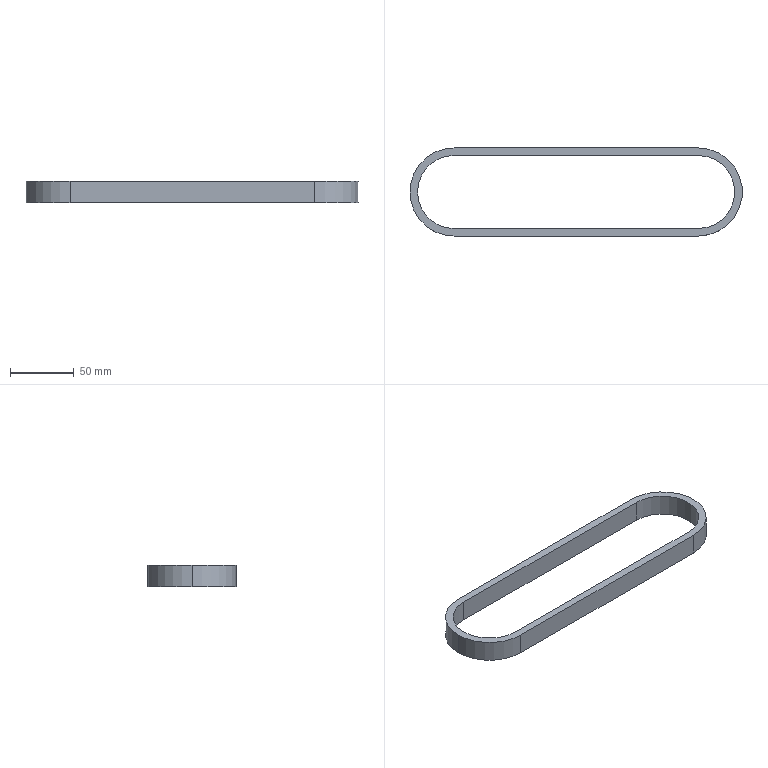Part | SolidWorks | features BaseBody 1 | 1 solid | 12 faces | box 259.87 x 68.87 x 17 mm | volume 58157 mm3 | cylinder 6 | plane 6 | commonest cylinder face diameters 57.07 x3 68.87 x3
STEP:
#1=CARTESIAN_POINT('',(0.,28.535,17.));
#2=VERTEX_POINT('',#1);
#3=CARTESIAN_POINT('',(-28.535,0.,17.));
#4=VERTEX_POINT('',#3);
#5=CARTESIAN_POINT('',(0.,0.,17.));
#6=DIRECTION('',(0.,0.,1.));
#7=DIRECTION('',(1.,0.,0.));
#8=AXIS2_PLACEMENT_3D('',#5,#6,#7);
#9=CIRCLE('',#8,28.535);
#10=EDGE_CURVE('',#2,#4,#9,.T.);
#11=ORIENTED_EDGE('',*,*,#10,.T.);
#12=CARTESIAN_POINT('',(-28.535,0.,0.));
#13=VERTEX_POINT('',#12);
#14=CARTESIAN_POINT('',(-28.535,0.,17.));
#15=DIRECTION('',(0.,0.,-1.));
#16=VECTOR('',#15,1000.);
#17=LINE('',#14,#16);
#18=EDGE_CURVE('',#4,#13,#17,.T.);
#19=ORIENTED_EDGE('',*,*,#18,.T.);
#20=CARTESIAN_POINT('',(0.,28.535,0.));
#21=VERTEX_POINT('',#20);
#22=CARTESIAN_POINT('',(0.,0.,0.));
#23=DIRECTION('',(0.,0.,1.));
#24=DIRECTION('',(1.,0.,0.));
#25=AXIS2_PLACEMENT_3D('',#22,#23,#24);
#26=CIRCLE('',#25,28.535);
#27=EDGE_CURVE('',#21,#13,#26,.T.);
#28=ORIENTED_EDGE('',*,*,#27,.F.);
#29=CARTESIAN_POINT('',(0.,28.535,17.));
#30=DIRECTION('',(0.,0.,-1.));
#31=VECTOR('',#30,1000.);
#32=LINE('',#29,#31);
#33=EDGE_CURVE('',#2,#21,#32,.T.);
#34=ORIENTED_EDGE('',*,*,#33,.F.);
#35=EDGE_LOOP('',(#11,#19,#28,#34));
#36=FACE_OUTER_BOUND('',#35,.T.);
#37=CARTESIAN_POINT('',(0.,0.,17.));
#38=DIRECTION('',(0.,0.,-1.));
#39=DIRECTION('',(-1.,0.,0.));
#40=AXIS2_PLACEMENT_3D('',#37,#38,#39);
#41=CYLINDRICAL_SURFACE('',#40,28.535);
#42=ADVANCED_FACE('',(#36),#41,.F.);
#43=CARTESIAN_POINT('',(-34.435,0.,17.));
#44=VERTEX_POINT('',#43);
#45=CARTESIAN_POINT('',(0.,-34.435,17.));
#46=VERTEX_POINT('',#45);
#47=CARTESIAN_POINT('',(0.,0.,17.));
#48=DIRECTION('',(0.,0.,1.));
#49=DIRECTION('',(1.,0.,0.));
#50=AXIS2_PLACEMENT_3D('',#47,#48,#49);
#51=CIRCLE('',#50,34.435);
#52=EDGE_CURVE('',#44,#46,#51,.T.);
#53=ORIENTED_EDGE('',*,*,#52,.F.);
#54=CARTESIAN_POINT('',(-34.435,0.,0.));
#55=VERTEX_POINT('',#54);
#56=CARTESIAN_POINT('',(-34.435,0.,17.));
#57=DIRECTION('',(0.,0.,-1.));
#58=VECTOR('',#57,1000.);
#59=LINE('',#56,#58);
#60=EDGE_CURVE('',#44,#55,#59,.T.);
#61=ORIENTED_EDGE('',*,*,#60,.T.);
#62=CARTESIAN_POINT('',(0.,-34.435,0.));
#63=VERTEX_POINT('',#62);
#64=CARTESIAN_POINT('',(0.,0.,0.));
#65=DIRECTION('',(0.,0.,1.));
#66=DIRECTION('',(1.,0.,0.));
#67=AXIS2_PLACEMENT_3D('',#64,#65,#66);
#68=CIRCLE('',#67,34.435);
#69=EDGE_CURVE('',#55,#63,#68,.T.);
#70=ORIENTED_EDGE('',*,*,#69,.T.);
#71=CARTESIAN_POINT('',(0.,-34.435,17.));
#72=DIRECTION('',(0.,0.,-1.));
#73=VECTOR('',#72,1000.);
#74=LINE('',#71,#73);
#75=EDGE_CURVE('',#46,#63,#74,.T.);
#76=ORIENTED_EDGE('',*,*,#75,.F.);
#77=EDGE_LOOP('',(#53,#61,#70,#76));
#78=FACE_OUTER_BOUND('',#77,.T.);
#79=CARTESIAN_POINT('',(0.,0.,17.));
#80=DIRECTION('',(0.,0.,-1.));
#81=DIRECTION('',(-1.,0.,0.));
#82=AXIS2_PLACEMENT_3D('',#79,#80,#81);
#83=CYLINDRICAL_SURFACE('',#82,34.435);
#84=ADVANCED_FACE('',(#78),#83,.T.);
#85=CARTESIAN_POINT('',(0.,34.435,17.));
#86=VERTEX_POINT('',#85);
#87=CARTESIAN_POINT('',(0.,0.,17.));
#88=DIRECTION('',(0.,0.,1.));
#89=DIRECTION('',(1.,0.,0.));
#90=AXIS2_PLACEMENT_3D('',#87,#88,#89);
#91=CIRCLE('',#90,34.435);
#92=EDGE_CURVE('',#86,#44,#91,.T.);
#93=ORIENTED_EDGE('',*,*,#92,.T.);
#94=ORIENTED_EDGE('',*,*,#52,.T.);
#95=CARTESIAN_POINT('',(191.,-34.435,17.));
#96=VERTEX_POINT('',#95);
#97=CARTESIAN_POINT('',(0.,-34.435,17.));
#98=DIRECTION('',(1.,0.,0.));
#99=VECTOR('',#98,1000.);
#100=LINE('',#97,#99);
#101=EDGE_CURVE('',#46,#96,#100,.T.);
#102=ORIENTED_EDGE('',*,*,#101,.T.);
#103=CARTESIAN_POINT('',(191.,34.435,17.));
#104=VERTEX_POINT('',#103);
#105=CARTESIAN_POINT('',(191.,0.,17.));
#106=DIRECTION('',(0.,0.,1.));
#107=DIRECTION('',(1.,0.,0.));
#108=AXIS2_PLACEMENT_3D('',#105,#106,#107);
#109=CIRCLE('',#108,34.435);
#110=EDGE_CURVE('',#96,#104,#109,.T.);
#111=ORIENTED_EDGE('',*,*,#110,.T.);
#112=CARTESIAN_POINT('',(0.,34.435,17.));
#113=DIRECTION('',(-1.,0.,0.));
#114=VECTOR('',#113,1000.);
#115=LINE('',#112,#114);
#116=EDGE_CURVE('',#104,#86,#115,.T.);
#117=ORIENTED_EDGE('',*,*,#116,.T.);
#118=EDGE_LOOP('',(#93,#94,#102,#111,#117));
#119=FACE_OUTER_BOUND('',#118,.T.);
#120=CARTESIAN_POINT('',(0.,-28.535,17.));
#121=VERTEX_POINT('',#120);
#122=CARTESIAN_POINT('',(191.,-28.535,17.));
#123=VERTEX_POINT('',#122);
#124=CARTESIAN_POINT('',(0.,-28.535,17.));
#125=DIRECTION('',(1.,0.,0.));
#126=VECTOR('',#125,1000.);
#127=LINE('',#124,#126);
#128=EDGE_CURVE('',#121,#123,#127,.T.);
#129=ORIENTED_EDGE('',*,*,#128,.F.);
#130=CARTESIAN_POINT('',(0.,0.,17.));
#131=DIRECTION('',(0.,0.,1.));
#132=DIRECTION('',(1.,0.,0.));
#133=AXIS2_PLACEMENT_3D('',#130,#131,#132);
#134=CIRCLE('',#133,28.535);
#135=EDGE_CURVE('',#4,#121,#134,.T.);
#136=ORIENTED_EDGE('',*,*,#135,.F.);
#137=ORIENTED_EDGE('',*,*,#10,.F.);
#138=CARTESIAN_POINT('',(191.,28.535,17.));
#139=VERTEX_POINT('',#138);
#140=CARTESIAN_POINT('',(0.,28.535,17.));
#141=DIRECTION('',(-1.,0.,0.));
#142=VECTOR('',#141,1000.);
#143=LINE('',#140,#142);
#144=EDGE_CURVE('',#139,#2,#143,.T.);
#145=ORIENTED_EDGE('',*,*,#144,.F.);
#146=CARTESIAN_POINT('',(191.,0.,17.));
#147=DIRECTION('',(0.,0.,1.));
#148=DIRECTION('',(1.,0.,0.));
#149=AXIS2_PLACEMENT_3D('',#146,#147,#148);
#150=CIRCLE('',#149,28.535);
#151=EDGE_CURVE('',#123,#139,#150,.T.);
#152=ORIENTED_EDGE('',*,*,#151,.F.);
#153=EDGE_LOOP('',(#129,#136,#137,#145,#152));
#154=FACE_BOUND('',#153,.T.);
#155=CARTESIAN_POINT('',(0.,0.,17.));
#156=DIRECTION('',(0.,0.,1.));
#157=DIRECTION('',(1.,0.,0.));
#158=AXIS2_PLACEMENT_3D('',#155,#156,#157);
#159=PLANE('',#158);
#160=ADVANCED_FACE('',(#119,#154),#159,.T.);
#161=CARTESIAN_POINT('',(0.,34.435,0.));
#162=VERTEX_POINT('',#161);
#163=CARTESIAN_POINT('',(0.,0.,0.));
#164=DIRECTION('',(0.,0.,1.));
#165=DIRECTION('',(1.,0.,0.));
#166=AXIS2_PLACEMENT_3D('',#163,#164,#165);
#167=CIRCLE('',#166,34.435);
#168=EDGE_CURVE('',#162,#55,#167,.T.);
#169=ORIENTED_EDGE('',*,*,#168,.F.);
#170=CARTESIAN_POINT('',(191.,34.435,0.));
#171=VERTEX_POINT('',#170);
#172=CARTESIAN_POINT('',(0.,34.435,0.));
#173=DIRECTION('',(-1.,0.,0.));
#174=VECTOR('',#173,1000.);
#175=LINE('',#172,#174);
#176=EDGE_CURVE('',#171,#162,#175,.T.);
#177=ORIENTED_EDGE('',*,*,#176,.F.);
#178=CARTESIAN_POINT('',(191.,-34.435,0.));
#179=VERTEX_POINT('',#178);
#180=CARTESIAN_POINT('',(191.,0.,0.));
#181=DIRECTION('',(0.,0.,1.));
#182=DIRECTION('',(1.,0.,0.));
#183=AXIS2_PLACEMENT_3D('',#180,#181,#182);
#184=CIRCLE('',#183,34.435);
#185=EDGE_CURVE('',#179,#171,#184,.T.);
#186=ORIENTED_EDGE('',*,*,#185,.F.);
#187=CARTESIAN_POINT('',(0.,-34.435,0.));
#188=DIRECTION('',(1.,0.,0.));
#189=VECTOR('',#188,1000.);
#190=LINE('',#187,#189);
#191=EDGE_CURVE('',#63,#179,#190,.T.);
#192=ORIENTED_EDGE('',*,*,#191,.F.);
#193=ORIENTED_EDGE('',*,*,#69,.F.);
#194=EDGE_LOOP('',(#169,#177,#186,#192,#193));
#195=FACE_OUTER_BOUND('',#194,.T.);
#196=ORIENTED_EDGE('',*,*,#27,.T.);
#197=CARTESIAN_POINT('',(0.,-28.535,0.));
#198=VERTEX_POINT('',#197);
#199=CARTESIAN_POINT('',(0.,0.,0.));
#200=DIRECTION('',(0.,0.,1.));
#201=DIRECTION('',(1.,0.,0.));
#202=AXIS2_PLACEMENT_3D('',#199,#200,#201);
#203=CIRCLE('',#202,28.535);
#204=EDGE_CURVE('',#13,#198,#203,.T.);
#205=ORIENTED_EDGE('',*,*,#204,.T.);
#206=CARTESIAN_POINT('',(191.,-28.535,0.));
#207=VERTEX_POINT('',#206);
#208=CARTESIAN_POINT('',(0.,-28.535,0.));
#209=DIRECTION('',(1.,0.,0.));
#210=VECTOR('',#209,1000.);
#211=LINE('',#208,#210);
#212=EDGE_CURVE('',#198,#207,#211,.T.);
#213=ORIENTED_EDGE('',*,*,#212,.T.);
#214=CARTESIAN_POINT('',(191.,28.535,0.));
#215=VERTEX_POINT('',#214);
#216=CARTESIAN_POINT('',(191.,0.,0.));
#217=DIRECTION('',(0.,0.,1.));
#218=DIRECTION('',(1.,0.,0.));
#219=AXIS2_PLACEMENT_3D('',#216,#217,#218);
#220=CIRCLE('',#219,28.535);
#221=EDGE_CURVE('',#207,#215,#220,.T.);
#222=ORIENTED_EDGE('',*,*,#221,.T.);
#223=CARTESIAN_POINT('',(0.,28.535,0.));
#224=DIRECTION('',(-1.,0.,0.));
#225=VECTOR('',#224,1000.);
#226=LINE('',#223,#225);
#227=EDGE_CURVE('',#215,#21,#226,.T.);
#228=ORIENTED_EDGE('',*,*,#227,.T.);
#229=EDGE_LOOP('',(#196,#205,#213,#222,#228));
#230=FACE_BOUND('',#229,.T.);
#231=CARTESIAN_POINT('',(0.,0.,0.));
#232=DIRECTION('',(0.,0.,1.));
#233=DIRECTION('',(1.,0.,0.));
#234=AXIS2_PLACEMENT_3D('',#231,#232,#233);
#235=PLANE('',#234);
#236=ADVANCED_FACE('',(#195,#230),#235,.F.);
#237=ORIENTED_EDGE('',*,*,#60,.F.);
#238=ORIENTED_EDGE('',*,*,#92,.F.);
#239=CARTESIAN_POINT('',(0.,34.435,17.));
#240=DIRECTION('',(0.,0.,-1.));
#241=VECTOR('',#240,1000.);
#242=LINE('',#239,#241);
#243=EDGE_CURVE('',#86,#162,#242,.T.);
#244=ORIENTED_EDGE('',*,*,#243,.T.);
#245=ORIENTED_EDGE('',*,*,#168,.T.);
#246=EDGE_LOOP('',(#237,#238,#244,#245));
#247=FACE_OUTER_BOUND('',#246,.T.);
#248=CARTESIAN_POINT('',(0.,0.,17.));
#249=DIRECTION('',(0.,0.,-1.));
#250=DIRECTION('',(-1.,0.,0.));
#251=AXIS2_PLACEMENT_3D('',#248,#249,#250);
#252=CYLINDRICAL_SURFACE('',#251,34.435);
#253=ADVANCED_FACE('',(#247),#252,.T.);
#254=ORIENTED_EDGE('',*,*,#191,.T.);
#255=CARTESIAN_POINT('',(191.,-34.435,17.));
#256=DIRECTION('',(0.,0.,-1.));
#257=VECTOR('',#256,1000.);
#258=LINE('',#255,#257);
#259=EDGE_CURVE('',#96,#179,#258,.T.);
#260=ORIENTED_EDGE('',*,*,#259,.F.);
#261=ORIENTED_EDGE('',*,*,#101,.F.);
#262=ORIENTED_EDGE('',*,*,#75,.T.);
#263=EDGE_LOOP('',(#254,#260,#261,#262));
#264=FACE_OUTER_BOUND('',#263,.T.);
#265=CARTESIAN_POINT('',(0.,-34.435,17.));
#266=DIRECTION('',(0.,1.,0.));
#267=DIRECTION('',(0.,0.,1.));
#268=AXIS2_PLACEMENT_3D('',#265,#266,#267);
#269=PLANE('',#268);
#270=ADVANCED_FACE('',(#264),#269,.F.);
#271=ORIENTED_EDGE('',*,*,#185,.T.);
#272=CARTESIAN_POINT('',(191.,34.435,17.));
#273=DIRECTION('',(0.,0.,-1.));
#274=VECTOR('',#273,1000.);
#275=LINE('',#272,#274);
#276=EDGE_CURVE('',#104,#171,#275,.T.);
#277=ORIENTED_EDGE('',*,*,#276,.F.);
#278=ORIENTED_EDGE('',*,*,#110,.F.);
#279=ORIENTED_EDGE('',*,*,#259,.T.);
#280=EDGE_LOOP('',(#271,#277,#278,#279));
#281=FACE_OUTER_BOUND('',#280,.T.);
#282=CARTESIAN_POINT('',(191.,0.,17.));
#283=DIRECTION('',(0.,0.,-1.));
#284=DIRECTION('',(-1.,0.,0.));
#285=AXIS2_PLACEMENT_3D('',#282,#283,#284);
#286=CYLINDRICAL_SURFACE('',#285,34.435);
#287=ADVANCED_FACE('',(#281),#286,.T.);
#288=ORIENTED_EDGE('',*,*,#176,.T.);
#289=ORIENTED_EDGE('',*,*,#243,.F.);
#290=ORIENTED_EDGE('',*,*,#116,.F.);
#291=ORIENTED_EDGE('',*,*,#276,.T.);
#292=EDGE_LOOP('',(#288,#289,#290,#291));
#293=FACE_OUTER_BOUND('',#292,.T.);
#294=CARTESIAN_POINT('',(0.,34.435,17.));
#295=DIRECTION('',(0.,-1.,0.));
#296=DIRECTION('',(0.,0.,-1.));
#297=AXIS2_PLACEMENT_3D('',#294,#295,#296);
#298=PLANE('',#297);
#299=ADVANCED_FACE('',(#293),#298,.F.);
#300=ORIENTED_EDGE('',*,*,#18,.F.);
#301=ORIENTED_EDGE('',*,*,#135,.T.);
#302=CARTESIAN_POINT('',(0.,-28.535,17.));
#303=DIRECTION('',(0.,0.,-1.));
#304=VECTOR('',#303,1000.);
#305=LINE('',#302,#304);
#306=EDGE_CURVE('',#121,#198,#305,.T.);
#307=ORIENTED_EDGE('',*,*,#306,.T.);
#308=ORIENTED_EDGE('',*,*,#204,.F.);
#309=EDGE_LOOP('',(#300,#301,#307,#308));
#310=FACE_OUTER_BOUND('',#309,.T.);
#311=CARTESIAN_POINT('',(0.,0.,17.));
#312=DIRECTION('',(0.,0.,-1.));
#313=DIRECTION('',(-1.,0.,0.));
#314=AXIS2_PLACEMENT_3D('',#311,#312,#313);
#315=CYLINDRICAL_SURFACE('',#314,28.535);
#316=ADVANCED_FACE('',(#310),#315,.F.);
#317=ORIENTED_EDGE('',*,*,#212,.F.);
#318=ORIENTED_EDGE('',*,*,#306,.F.);
#319=ORIENTED_EDGE('',*,*,#128,.T.);
#320=CARTESIAN_POINT('',(191.,-28.535,17.));
#321=DIRECTION('',(0.,0.,-1.));
#322=VECTOR('',#321,1000.);
#323=LINE('',#320,#322);
#324=EDGE_CURVE('',#123,#207,#323,.T.);
#325=ORIENTED_EDGE('',*,*,#324,.T.);
#326=EDGE_LOOP('',(#317,#318,#319,#325));
#327=FACE_OUTER_BOUND('',#326,.T.);
#328=CARTESIAN_POINT('',(0.,-28.535,17.));
#329=DIRECTION('',(0.,1.,0.));
#330=DIRECTION('',(-1.,0.,0.));
#331=AXIS2_PLACEMENT_3D('',#328,#329,#330);
#332=PLANE('',#331);
#333=ADVANCED_FACE('',(#327),#332,.T.);
#334=ORIENTED_EDGE('',*,*,#221,.F.);
#335=ORIENTED_EDGE('',*,*,#324,.F.);
#336=ORIENTED_EDGE('',*,*,#151,.T.);
#337=CARTESIAN_POINT('',(191.,28.535,17.));
#338=DIRECTION('',(0.,0.,-1.));
#339=VECTOR('',#338,1000.);
#340=LINE('',#337,#339);
#341=EDGE_CURVE('',#139,#215,#340,.T.);
#342=ORIENTED_EDGE('',*,*,#341,.T.);
#343=EDGE_LOOP('',(#334,#335,#336,#342));
#344=FACE_OUTER_BOUND('',#343,.T.);
#345=CARTESIAN_POINT('',(191.,0.,17.));
#346=DIRECTION('',(0.,0.,-1.));
#347=DIRECTION('',(-1.,0.,0.));
#348=AXIS2_PLACEMENT_3D('',#345,#346,#347);
#349=CYLINDRICAL_SURFACE('',#348,28.535);
#350=ADVANCED_FACE('',(#344),#349,.F.);
#351=ORIENTED_EDGE('',*,*,#227,.F.);
#352=ORIENTED_EDGE('',*,*,#341,.F.);
#353=ORIENTED_EDGE('',*,*,#144,.T.);
#354=ORIENTED_EDGE('',*,*,#33,.T.);
#355=EDGE_LOOP('',(#351,#352,#353,#354));
#356=FACE_OUTER_BOUND('',#355,.T.);
#357=CARTESIAN_POINT('',(0.,28.535,17.));
#358=DIRECTION('',(0.,-1.,0.));
#359=DIRECTION('',(1.,0.,0.));
#360=AXIS2_PLACEMENT_3D('',#357,#358,#359);
#361=PLANE('',#360);
#362=ADVANCED_FACE('',(#356),#361,.T.);
#363=CLOSED_SHELL('',(#42,#84,#160,#236,#253,#270,#287,#299,#316,#333,#350,#362));
#364=MANIFOLD_SOLID_BREP('',#363);
#365=CARTESIAN_POINT('',(0.,0.,0.));
#366=DIRECTION('',(0.,0.,1.));
#367=DIRECTION('',(1.,0.,0.));
#368=AXIS2_PLACEMENT_3D('',#365,#366,#367);
#369=(LENGTH_UNIT()NAMED_UNIT(*)SI_UNIT(.MILLI.,.METRE.));
#370=UNCERTAINTY_MEASURE_WITH_UNIT(LENGTH_MEASURE(0.00001),#369,'','');
#371=(NAMED_UNIT(*)PLANE_ANGLE_UNIT()SI_UNIT($,.RADIAN.));
#372=(NAMED_UNIT(*)SI_UNIT($,.STERADIAN.)SOLID_ANGLE_UNIT());
#373=(GEOMETRIC_REPRESENTATION_CONTEXT(3)GLOBAL_UNCERTAINTY_ASSIGNED_CONTEXT((#370))GLOBAL_UNIT_ASSIGNED_CONTEXT((#369,#371,#372))REPRESENTATION_CONTEXT('',''));
#374=ADVANCED_BREP_SHAPE_REPRESENTATION('',(#364,#368),#373);